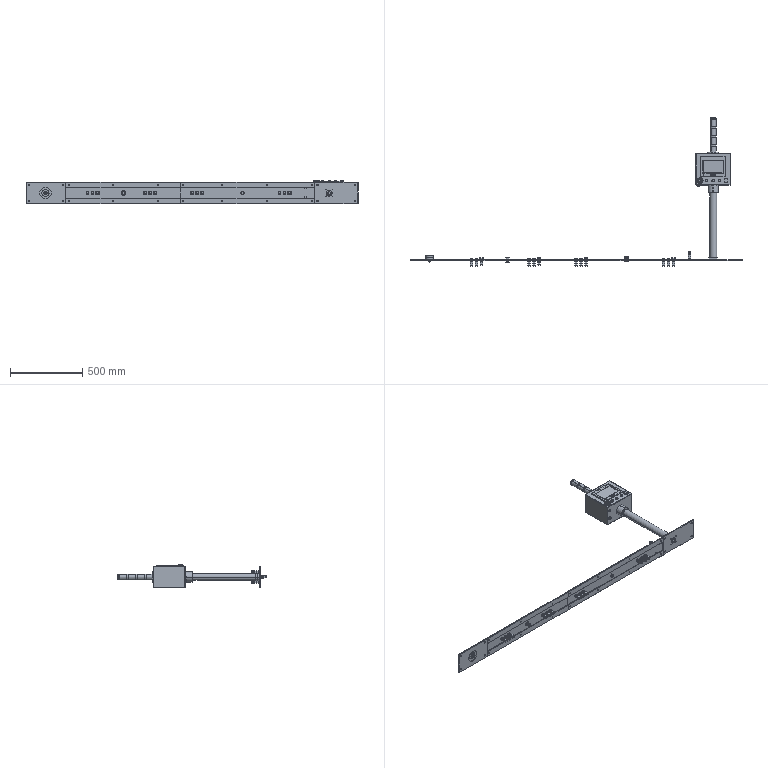Part | NX | 55 solids | 3165 faces | volume 4087606 mm3 | plane 2180 | cylinder 796 | cone 120 | torus 46 | spline 12 | sphere 11 | commonest cylinder face diameters 1 x96 7 x72 21 x72 15.6 x64 16 x50 18 x43